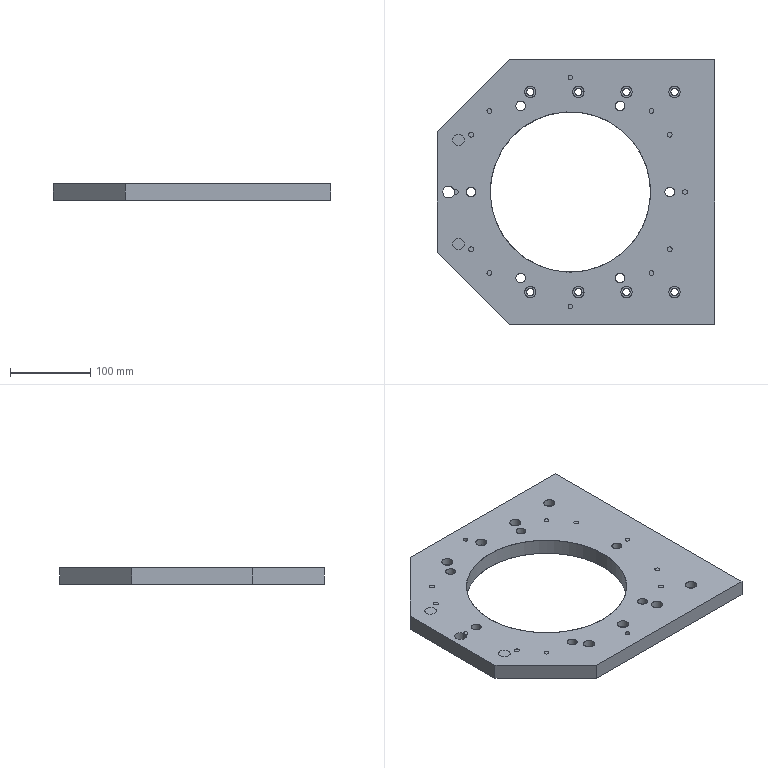Part | 2 solids | 118 faces | box 346 x 330 x 20 mm | volume 2905785 mm3 | cylinder 68 | plane 38 | cone 12 | commonest cylinder face diameters 9 x16 14 x16 6 x14 12 x12 6.8 x4 14.5 x4